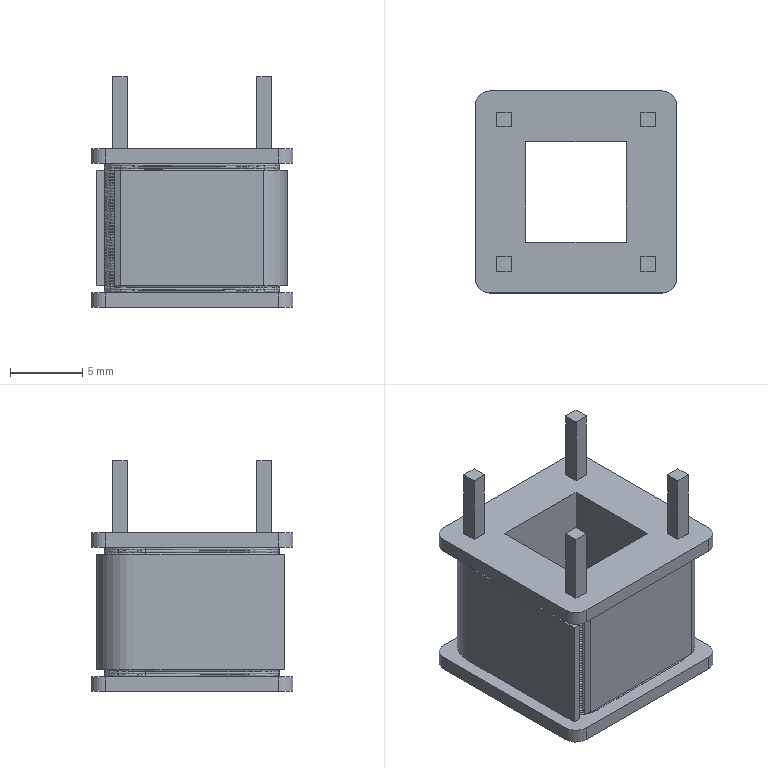Part | NX | features BREP 46, LINKED_BODY 1 | 47 solids | 240 faces | box 14 x 14 x 16 mm | volume 921.369 mm3 | spline 183 | plane 45 | cylinder 12 | commonest cylinder face diameters 2 x12